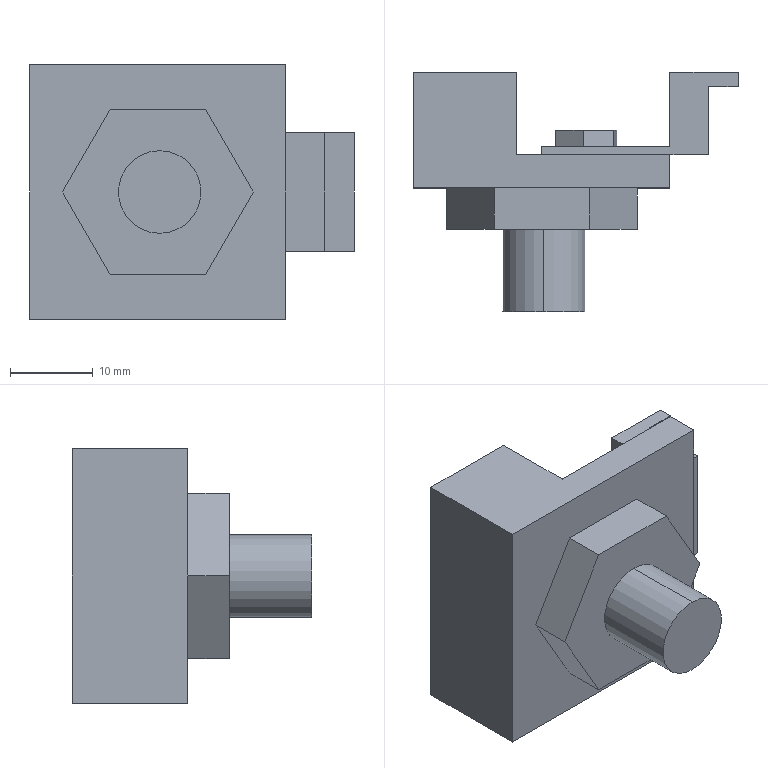Part | SolidWorks | features ICE 9, Extrusion 1 | 1 solid | 54 faces | box 39.277 x 29 x 30.752 mm | volume 9979 mm3 | plane 46 | cylinder 8 | commonest cylinder face diameters 8.542 x4 3.886 x2 10 x2
STEP:
#1=CARTESIAN_POINT('',(19.89,18.9,-1.943));
#2=VERTEX_POINT('',#1);
#3=CARTESIAN_POINT('',(18.72,18.9,1.551));
#4=VERTEX_POINT('',#3);
#5=CARTESIAN_POINT('',(19.89,18.9,0.));
#6=DIRECTION('',(0.,1.,0.));
#7=DIRECTION('',(0.,0.,1.));
#8=AXIS2_PLACEMENT_3D('',#5,#6,#7);
#9=CIRCLE('',#8,1.943);
#10=EDGE_CURVE('',#2,#4,#9,.T.);
#11=ORIENTED_EDGE('',*,*,#10,.F.);
#12=CARTESIAN_POINT('',(19.89,19.,-1.943));
#13=VERTEX_POINT('',#12);
#14=CARTESIAN_POINT('',(19.89,18.9,-1.943));
#15=DIRECTION('',(0.,1.,0.));
#16=VECTOR('',#15,1000.);
#17=LINE('',#14,#16);
#18=EDGE_CURVE('',#2,#13,#17,.T.);
#19=ORIENTED_EDGE('',*,*,#18,.T.);
#20=CARTESIAN_POINT('',(19.89,19.,1.943));
#21=VERTEX_POINT('',#20);
#22=CARTESIAN_POINT('',(19.89,19.,0.));
#23=DIRECTION('',(0.,1.,0.));
#24=DIRECTION('',(0.,0.,1.));
#25=AXIS2_PLACEMENT_3D('',#22,#23,#24);
#26=CIRCLE('',#25,1.943);
#27=EDGE_CURVE('',#13,#21,#26,.T.);
#28=ORIENTED_EDGE('',*,*,#27,.T.);
#29=CARTESIAN_POINT('',(19.89,18.9,1.943));
#30=VERTEX_POINT('',#29);
#31=CARTESIAN_POINT('',(19.89,18.9,1.943));
#32=DIRECTION('',(0.,1.,0.));
#33=VECTOR('',#32,1000.);
#34=LINE('',#31,#33);
#35=EDGE_CURVE('',#30,#21,#34,.T.);
#36=ORIENTED_EDGE('',*,*,#35,.F.);
#37=CARTESIAN_POINT('',(19.07,18.9,1.762));
#38=VERTEX_POINT('',#37);
#39=CARTESIAN_POINT('',(19.89,18.9,0.));
#40=DIRECTION('',(0.,1.,0.));
#41=DIRECTION('',(0.,0.,1.));
#42=AXIS2_PLACEMENT_3D('',#39,#40,#41);
#43=CIRCLE('',#42,1.943);
#44=EDGE_CURVE('',#38,#30,#43,.T.);
#45=ORIENTED_EDGE('',*,*,#44,.F.);
#46=CARTESIAN_POINT('',(18.89,18.9,1.666));
#47=VERTEX_POINT('',#46);
#48=CARTESIAN_POINT('',(19.89,18.9,0.));
#49=DIRECTION('',(0.,1.,0.));
#50=DIRECTION('',(0.,0.,1.));
#51=AXIS2_PLACEMENT_3D('',#48,#49,#50);
#52=CIRCLE('',#51,1.943);
#53=EDGE_CURVE('',#47,#38,#52,.T.);
#54=ORIENTED_EDGE('',*,*,#53,.F.);
#55=CARTESIAN_POINT('',(19.89,18.9,0.));
#56=DIRECTION('',(0.,1.,0.));
#57=DIRECTION('',(0.,0.,1.));
#58=AXIS2_PLACEMENT_3D('',#55,#56,#57);
#59=CIRCLE('',#58,1.943);
#60=EDGE_CURVE('',#4,#47,#59,.T.);
#61=ORIENTED_EDGE('',*,*,#60,.F.);
#62=EDGE_LOOP('',(#11,#19,#28,#36,#45,#54,#61));
#63=FACE_OUTER_BOUND('',#62,.T.);
#64=CARTESIAN_POINT('',(19.89,18.9,0.));
#65=DIRECTION('',(0.,1.,0.));
#66=DIRECTION('',(0.,0.,1.));
#67=AXIS2_PLACEMENT_3D('',#64,#65,#66);
#68=CYLINDRICAL_SURFACE('',#67,1.943);
#69=ADVANCED_FACE('',(#63),#68,.F.);
#70=CARTESIAN_POINT('',(-9.584,8.,-10.188));
#71=VERTEX_POINT('',#70);
#72=CARTESIAN_POINT('',(-9.584,8.,-1.646));
#73=VERTEX_POINT('',#72);
#74=CARTESIAN_POINT('',(-9.584,8.,-5.917));
#75=DIRECTION('',(0.,1.,0.));
#76=DIRECTION('',(0.,0.,1.));
#77=AXIS2_PLACEMENT_3D('',#74,#75,#76);
#78=CIRCLE('',#77,4.271);
#79=EDGE_CURVE('',#71,#73,#78,.T.);
#80=ORIENTED_EDGE('',*,*,#79,.F.);
#81=CARTESIAN_POINT('',(-9.584,19.,-10.188));
#82=VERTEX_POINT('',#81);
#83=CARTESIAN_POINT('',(-9.584,8.,-10.188));
#84=DIRECTION('',(0.,1.,0.));
#85=VECTOR('',#84,1000.);
#86=LINE('',#83,#85);
#87=EDGE_CURVE('',#71,#82,#86,.T.);
#88=ORIENTED_EDGE('',*,*,#87,.T.);
#89=CARTESIAN_POINT('',(-9.584,19.,-1.646));
#90=VERTEX_POINT('',#89);
#91=CARTESIAN_POINT('',(-9.584,19.,-5.917));
#92=DIRECTION('',(0.,1.,0.));
#93=DIRECTION('',(0.,0.,1.));
#94=AXIS2_PLACEMENT_3D('',#91,#92,#93);
#95=CIRCLE('',#94,4.271);
#96=EDGE_CURVE('',#82,#90,#95,.T.);
#97=ORIENTED_EDGE('',*,*,#96,.T.);
#98=CARTESIAN_POINT('',(-9.584,8.,-1.646));
#99=DIRECTION('',(0.,1.,0.));
#100=VECTOR('',#99,1000.);
#101=LINE('',#98,#100);
#102=EDGE_CURVE('',#73,#90,#101,.T.);
#103=ORIENTED_EDGE('',*,*,#102,.F.);
#104=EDGE_LOOP('',(#80,#88,#97,#103));
#105=FACE_OUTER_BOUND('',#104,.T.);
#106=CARTESIAN_POINT('',(-9.584,8.,-5.917));
#107=DIRECTION('',(0.,1.,0.));
#108=DIRECTION('',(0.,0.,1.));
#109=AXIS2_PLACEMENT_3D('',#106,#107,#108);
#110=CYLINDRICAL_SURFACE('',#109,4.271);
#111=ADVANCED_FACE('',(#105),#110,.F.);
#112=CARTESIAN_POINT('',(-9.584,8.,2.375));
#113=VERTEX_POINT('',#112);
#114=CARTESIAN_POINT('',(-9.584,8.,10.916));
#115=VERTEX_POINT('',#114);
#116=CARTESIAN_POINT('',(-9.584,8.,6.646));
#117=DIRECTION('',(0.,1.,0.));
#118=DIRECTION('',(0.,0.,1.));
#119=AXIS2_PLACEMENT_3D('',#116,#117,#118);
#120=CIRCLE('',#119,4.271);
#121=EDGE_CURVE('',#113,#115,#120,.T.);
#122=ORIENTED_EDGE('',*,*,#121,.F.);
#123=CARTESIAN_POINT('',(-9.584,19.,2.375));
#124=VERTEX_POINT('',#123);
#125=CARTESIAN_POINT('',(-9.584,8.,2.375));
#126=DIRECTION('',(0.,1.,0.));
#127=VECTOR('',#126,1000.);
#128=LINE('',#125,#127);
#129=EDGE_CURVE('',#113,#124,#128,.T.);
#130=ORIENTED_EDGE('',*,*,#129,.T.);
#131=CARTESIAN_POINT('',(-9.584,19.,10.916));
#132=VERTEX_POINT('',#131);
#133=CARTESIAN_POINT('',(-9.584,19.,6.646));
#134=DIRECTION('',(0.,1.,0.));
#135=DIRECTION('',(0.,0.,1.));
#136=AXIS2_PLACEMENT_3D('',#133,#134,#135);
#137=CIRCLE('',#136,4.271);
#138=EDGE_CURVE('',#124,#132,#137,.T.);
#139=ORIENTED_EDGE('',*,*,#138,.T.);
#140=CARTESIAN_POINT('',(-9.584,8.,10.916));
#141=DIRECTION('',(0.,1.,0.));
#142=VECTOR('',#141,1000.);
#143=LINE('',#140,#142);
#144=EDGE_CURVE('',#115,#132,#143,.T.);
#145=ORIENTED_EDGE('',*,*,#144,.F.);
#146=EDGE_LOOP('',(#122,#130,#139,#145));
#147=FACE_OUTER_BOUND('',#146,.T.);
#148=CARTESIAN_POINT('',(-9.584,8.,6.646));
#149=DIRECTION('',(0.,1.,0.));
#150=DIRECTION('',(0.,0.,1.));
#151=AXIS2_PLACEMENT_3D('',#148,#149,#150);
#152=CYLINDRICAL_SURFACE('',#151,4.271);
#153=ADVANCED_FACE('',(#147),#152,.F.);
#154=CARTESIAN_POINT('',(0.2348,-10.,-5.));
#155=VERTEX_POINT('',#154);
#156=CARTESIAN_POINT('',(0.2348,-10.,5.));
#157=VERTEX_POINT('',#156);
#158=CARTESIAN_POINT('',(0.2348,-10.,0.));
#159=DIRECTION('',(0.,-1.,0.));
#160=DIRECTION('',(0.,0.,-1.));
#161=AXIS2_PLACEMENT_3D('',#158,#159,#160);
#162=CIRCLE('',#161,5.);
#163=EDGE_CURVE('',#155,#157,#162,.T.);
#164=ORIENTED_EDGE('',*,*,#163,.F.);
#165=CARTESIAN_POINT('',(0.2348,0.,-5.));
#166=VERTEX_POINT('',#165);
#167=CARTESIAN_POINT('',(0.2348,-10.,-5.));
#168=DIRECTION('',(0.,1.,0.));
#169=VECTOR('',#168,1000.);
#170=LINE('',#167,#169);
#171=EDGE_CURVE('',#155,#166,#170,.T.);
#172=ORIENTED_EDGE('',*,*,#171,.T.);
#173=CARTESIAN_POINT('',(0.2348,0.,5.));
#174=VERTEX_POINT('',#173);
#175=CARTESIAN_POINT('',(0.2348,0.,0.));
#176=DIRECTION('',(0.,-1.,0.));
#177=DIRECTION('',(0.,0.,-1.));
#178=AXIS2_PLACEMENT_3D('',#175,#176,#177);
#179=CIRCLE('',#178,5.);
#180=EDGE_CURVE('',#166,#174,#179,.T.);
#181=ORIENTED_EDGE('',*,*,#180,.T.);
#182=CARTESIAN_POINT('',(0.2348,-10.,5.));
#183=DIRECTION('',(0.,1.,0.));
#184=VECTOR('',#183,1000.);
#185=LINE('',#182,#184);
#186=EDGE_CURVE('',#157,#174,#185,.T.);
#187=ORIENTED_EDGE('',*,*,#186,.F.);
#188=EDGE_LOOP('',(#164,#172,#181,#187));
#189=FACE_OUTER_BOUND('',#188,.T.);
#190=CARTESIAN_POINT('',(0.2348,-10.,0.));
#191=DIRECTION('',(0.,1.,0.));
#192=DIRECTION('',(0.,0.,1.));
#193=AXIS2_PLACEMENT_3D('',#190,#191,#192);
#194=CYLINDRICAL_SURFACE('',#193,5.);
#195=ADVANCED_FACE('',(#189),#194,.T.);
#196=CARTESIAN_POINT('',(15.495,10.,-7.2));
#197=VERTEX_POINT('',#196);
#198=CARTESIAN_POINT('',(15.495,10.,7.2));
#199=VERTEX_POINT('',#198);
#200=CARTESIAN_POINT('',(15.495,10.,-19.428));
#201=DIRECTION('',(0.,0.,1.));
#202=VECTOR('',#201,1000.);
#203=LINE('',#200,#202);
#204=EDGE_CURVE('',#197,#199,#203,.T.);
#205=ORIENTED_EDGE('',*,*,#204,.F.);
#206=CARTESIAN_POINT('',(0.,10.,-7.2));
#207=VERTEX_POINT('',#206);
#208=CARTESIAN_POINT('',(0.,10.,-7.2));
#209=DIRECTION('',(-1.,0.,0.));
#210=VECTOR('',#209,1000.);
#211=LINE('',#208,#210);
#212=EDGE_CURVE('',#197,#207,#211,.T.);
#213=ORIENTED_EDGE('',*,*,#212,.T.);
#214=CARTESIAN_POINT('',(0.,10.,7.2));
#215=VERTEX_POINT('',#214);
#216=CARTESIAN_POINT('',(0.,10.,-7.2));
#217=DIRECTION('',(0.,0.,1.));
#218=VECTOR('',#217,1000.);
#219=LINE('',#216,#218);
#220=EDGE_CURVE('',#207,#215,#219,.T.);
#221=ORIENTED_EDGE('',*,*,#220,.T.);
#222=CARTESIAN_POINT('',(0.,10.,7.2));
#223=DIRECTION('',(1.,0.,0.));
#224=VECTOR('',#223,1000.);
#225=LINE('',#222,#224);
#226=EDGE_CURVE('',#215,#199,#225,.T.);
#227=ORIENTED_EDGE('',*,*,#226,.T.);
#228=EDGE_LOOP('',(#205,#213,#221,#227));
#229=FACE_OUTER_BOUND('',#228,.T.);
#230=CARTESIAN_POINT('',(5.703,10.,-4.089));
#231=VERTEX_POINT('',#230);
#232=CARTESIAN_POINT('',(1.991,10.,-2.341));
#233=VERTEX_POINT('',#232);
#234=CARTESIAN_POINT('',(5.703,10.,-4.089));
#235=DIRECTION('',(-0.9047,0.,0.426));
#236=VECTOR('',#235,1000.);
#237=LINE('',#234,#236);
#238=EDGE_CURVE('',#231,#233,#237,.T.);
#239=ORIENTED_EDGE('',*,*,#238,.F.);
#240=CARTESIAN_POINT('',(9.073,10.,-1.748));
#241=VERTEX_POINT('',#240);
#242=CARTESIAN_POINT('',(9.073,10.,-1.748));
#243=DIRECTION('',(-0.8213,0.,-0.5705));
#244=VECTOR('',#243,1000.);
#245=LINE('',#242,#244);
#246=EDGE_CURVE('',#241,#231,#245,.T.);
#247=ORIENTED_EDGE('',*,*,#246,.F.);
#248=CARTESIAN_POINT('',(8.731,10.,2.341));
#249=VERTEX_POINT('',#248);
#250=CARTESIAN_POINT('',(8.731,10.,2.341));
#251=DIRECTION('',(0.0834,0.,-0.9965));
#252=VECTOR('',#251,1000.);
#253=LINE('',#250,#252);
#254=EDGE_CURVE('',#249,#241,#253,.T.);
#255=ORIENTED_EDGE('',*,*,#254,.F.);
#256=CARTESIAN_POINT('',(5.019,10.,4.089));
#257=VERTEX_POINT('',#256);
#258=CARTESIAN_POINT('',(5.019,10.,4.089));
#259=DIRECTION('',(0.9047,0.,-0.426));
#260=VECTOR('',#259,1000.);
#261=LINE('',#258,#260);
#262=EDGE_CURVE('',#257,#249,#261,.T.);
#263=ORIENTED_EDGE('',*,*,#262,.F.);
#264=CARTESIAN_POINT('',(1.649,10.,1.748));
#265=VERTEX_POINT('',#264);
#266=CARTESIAN_POINT('',(1.649,10.,1.748));
#267=DIRECTION('',(0.8213,0.,0.5705));
#268=VECTOR('',#267,1000.);
#269=LINE('',#266,#268);
#270=EDGE_CURVE('',#265,#257,#269,.T.);
#271=ORIENTED_EDGE('',*,*,#270,.F.);
#272=CARTESIAN_POINT('',(1.991,10.,-2.341));
#273=DIRECTION('',(-0.0834,0.,0.9965));
#274=VECTOR('',#273,1000.);
#275=LINE('',#272,#274);
#276=EDGE_CURVE('',#233,#265,#275,.T.);
#277=ORIENTED_EDGE('',*,*,#276,.F.);
#278=EDGE_LOOP('',(#239,#247,#255,#263,#271,#277));
#279=FACE_BOUND('',#278,.T.);
#280=CARTESIAN_POINT('',(0.,10.,0.));
#281=DIRECTION('',(0.,1.,0.));
#282=DIRECTION('',(0.,0.,1.));
#283=AXIS2_PLACEMENT_3D('',#280,#281,#282);
#284=PLANE('',#283);
#285=ADVANCED_FACE('',(#229,#279),#284,.T.);
#286=CARTESIAN_POINT('',(20.709,18.9,-1.762));
#287=VERTEX_POINT('',#286);
#288=CARTESIAN_POINT('',(19.714,18.9,-0.1053));
#289=DIRECTION('',(-0.5147,0.,0.8574));
#290=VECTOR('',#289,1000.);
#291=LINE('',#288,#290);
#292=EDGE_CURVE('',#287,#4,#291,.T.);
#293=ORIENTED_EDGE('',*,*,#292,.F.);
#294=CARTESIAN_POINT('',(19.89,18.9,0.));
#295=DIRECTION('',(0.,1.,0.));
#296=DIRECTION('',(0.,0.,1.));
#297=AXIS2_PLACEMENT_3D('',#294,#295,#296);
#298=CIRCLE('',#297,1.943);
#299=EDGE_CURVE('',#287,#2,#298,.T.);
#300=ORIENTED_EDGE('',*,*,#299,.T.);
#301=ORIENTED_EDGE('',*,*,#10,.T.);
#302=EDGE_LOOP('',(#293,#300,#301));
#303=FACE_OUTER_BOUND('',#302,.T.);
#304=CARTESIAN_POINT('',(19.89,18.9,0.));
#305=DIRECTION('',(0.,1.,0.));
#306=DIRECTION('',(0.,0.,1.));
#307=AXIS2_PLACEMENT_3D('',#304,#305,#306);
#308=PLANE('',#307);
#309=ADVANCED_FACE('',(#303),#308,.T.);
#310=CARTESIAN_POINT('',(15.504,9.,-7.2));
#311=VERTEX_POINT('',#310);
#312=CARTESIAN_POINT('',(0.,9.,-7.2));
#313=VERTEX_POINT('',#312);
#314=CARTESIAN_POINT('',(0.,9.,-7.2));
#315=DIRECTION('',(-1.,0.,0.));
#316=VECTOR('',#315,1000.);
#317=LINE('',#314,#316);
#318=EDGE_CURVE('',#311,#313,#317,.T.);
#319=ORIENTED_EDGE('',*,*,#318,.F.);
#320=CARTESIAN_POINT('',(15.504,9.,-15.376));
#321=VERTEX_POINT('',#320);
#322=CARTESIAN_POINT('',(15.504,9.,15.376));
#323=DIRECTION('',(0.,0.,-1.));
#324=VECTOR('',#323,1000.);
#325=LINE('',#322,#324);
#326=EDGE_CURVE('',#311,#321,#325,.T.);
#327=ORIENTED_EDGE('',*,*,#326,.T.);
#328=CARTESIAN_POINT('',(-3.031,9.,-15.376));
#329=VERTEX_POINT('',#328);
#330=CARTESIAN_POINT('',(-15.504,9.,-15.376));
#331=DIRECTION('',(-1.,0.,0.));
#332=VECTOR('',#331,1000.);
#333=LINE('',#330,#332);
#334=EDGE_CURVE('',#321,#329,#333,.T.);
#335=ORIENTED_EDGE('',*,*,#334,.T.);
#336=CARTESIAN_POINT('',(-3.031,9.,15.376));
#337=VERTEX_POINT('',#336);
#338=CARTESIAN_POINT('',(-3.031,9.,-15.376));
#339=DIRECTION('',(0.,0.,-1.));
#340=VECTOR('',#339,1000.);
#341=LINE('',#338,#340);
#342=EDGE_CURVE('',#337,#329,#341,.T.);
#343=ORIENTED_EDGE('',*,*,#342,.F.);
#344=CARTESIAN_POINT('',(15.504,9.,15.376));
#345=VERTEX_POINT('',#344);
#346=CARTESIAN_POINT('',(-15.504,9.,15.376));
#347=DIRECTION('',(1.,0.,0.));
#348=VECTOR('',#347,1000.);
#349=LINE('',#346,#348);
#350=EDGE_CURVE('',#337,#345,#349,.T.);
#351=ORIENTED_EDGE('',*,*,#350,.T.);
#352=CARTESIAN_POINT('',(15.504,9.,7.2));
#353=VERTEX_POINT('',#352);
#354=CARTESIAN_POINT('',(15.504,9.,15.376));
#355=DIRECTION('',(0.,0.,-1.));
#356=VECTOR('',#355,1000.);
#357=LINE('',#354,#356);
#358=EDGE_CURVE('',#345,#353,#357,.T.);
#359=ORIENTED_EDGE('',*,*,#358,.T.);
#360=CARTESIAN_POINT('',(0.,9.,7.2));
#361=VERTEX_POINT('',#360);
#362=CARTESIAN_POINT('',(0.,9.,7.2));
#363=DIRECTION('',(1.,0.,0.));
#364=VECTOR('',#363,1000.);
#365=LINE('',#362,#364);
#366=EDGE_CURVE('',#361,#353,#365,.T.);
#367=ORIENTED_EDGE('',*,*,#366,.F.);
#368=CARTESIAN_POINT('',(0.,9.,-7.2));
#369=DIRECTION('',(0.,0.,1.));
#370=VECTOR('',#369,1000.);
#371=LINE('',#368,#370);
#372=EDGE_CURVE('',#313,#361,#371,.T.);
#373=ORIENTED_EDGE('',*,*,#372,.F.);
#374=EDGE_LOOP('',(#319,#327,#335,#343,#351,#359,#367,#373));
#375=FACE_OUTER_BOUND('',#374,.T.);
#376=CARTESIAN_POINT('',(0.,9.,0.));
#377=DIRECTION('',(0.,-1.,0.));
#378=DIRECTION('',(0.,0.,-1.));
#379=AXIS2_PLACEMENT_3D('',#376,#377,#378);
#380=PLANE('',#379);
#381=ADVANCED_FACE('',(#375),#380,.F.);
#382=CARTESIAN_POINT('',(11.547,0.,0.));
#383=VERTEX_POINT('',#382);
#384=CARTESIAN_POINT('',(5.774,0.,-10.));
#385=VERTEX_POINT('',#384);
#386=CARTESIAN_POINT('',(11.547,0.,0.));
#387=DIRECTION('',(-0.5,0.,-0.866));
#388=VECTOR('',#387,1000.);
#389=LINE('',#386,#388);
#390=EDGE_CURVE('',#383,#385,#389,.T.);
#391=ORIENTED_EDGE('',*,*,#390,.T.);
#392=CARTESIAN_POINT('',(5.774,5.,-10.));
#393=VERTEX_POINT('',#392);
#394=CARTESIAN_POINT('',(5.774,5.,-10.));
#395=DIRECTION('',(0.,-1.,0.));
#396=VECTOR('',#395,1000.);
#397=LINE('',#394,#396);
#398=EDGE_CURVE('',#393,#385,#397,.T.);
#399=ORIENTED_EDGE('',*,*,#398,.F.);
#400=CARTESIAN_POINT('',(11.547,5.,0.));
#401=VERTEX_POINT('',#400);
#402=CARTESIAN_POINT('',(11.547,5.,0.));
#403=DIRECTION('',(-0.5,0.,-0.866));
#404=VECTOR('',#403,1000.);
#405=LINE('',#402,#404);
#406=EDGE_CURVE('',#401,#393,#405,.T.);
#407=ORIENTED_EDGE('',*,*,#406,.F.);
#408=CARTESIAN_POINT('',(11.547,5.,0.));
#409=DIRECTION('',(0.,-1.,0.));
#410=VECTOR('',#409,1000.);
#411=LINE('',#408,#410);
#412=EDGE_CURVE('',#401,#383,#411,.T.);
#413=ORIENTED_EDGE('',*,*,#412,.T.);
#414=EDGE_LOOP('',(#391,#399,#407,#413));
#415=FACE_OUTER_BOUND('',#414,.T.);
#416=CARTESIAN_POINT('',(11.547,5.,0.));
#417=DIRECTION('',(-0.866,0.,0.5));
#418=DIRECTION('',(0.5,0.,0.866));
#419=AXIS2_PLACEMENT_3D('',#416,#417,#418);
#420=PLANE('',#419);
#421=ADVANCED_FACE('',(#415),#420,.F.);
#422=CARTESIAN_POINT('',(-5.774,0.,-10.));
#423=VERTEX_POINT('',#422);
#424=CARTESIAN_POINT('',(5.774,0.,-10.));
#425=DIRECTION('',(-1.,0.,0.));
#426=VECTOR('',#425,1000.);
#427=LINE('',#424,#426);
#428=EDGE_CURVE('',#385,#423,#427,.T.);
#429=ORIENTED_EDGE('',*,*,#428,.T.);
#430=CARTESIAN_POINT('',(-5.774,5.,-10.));
#431=VERTEX_POINT('',#430);
#432=CARTESIAN_POINT('',(-5.774,5.,-10.));
#433=DIRECTION('',(0.,-1.,0.));
#434=VECTOR('',#433,1000.);
#435=LINE('',#432,#434);
#436=EDGE_CURVE('',#431,#423,#435,.T.);
#437=ORIENTED_EDGE('',*,*,#436,.F.);
#438=CARTESIAN_POINT('',(5.774,5.,-10.));
#439=DIRECTION('',(-1.,0.,0.));
#440=VECTOR('',#439,1000.);
#441=LINE('',#438,#440);
#442=EDGE_CURVE('',#393,#431,#441,.T.);
#443=ORIENTED_EDGE('',*,*,#442,.F.);
#444=ORIENTED_EDGE('',*,*,#398,.T.);
#445=EDGE_LOOP('',(#429,#437,#443,#444));
#446=FACE_OUTER_BOUND('',#445,.T.);
#447=CARTESIAN_POINT('',(5.774,5.,-10.));
#448=DIRECTION('',(0.,0.,1.));
#449=DIRECTION('',(1.,0.,0.));
#450=AXIS2_PLACEMENT_3D('',#447,#448,#449);
#451=PLANE('',#450);
#452=ADVANCED_FACE('',(#446),#451,.F.);
#453=CARTESIAN_POINT('',(-11.547,0.,0.));
#454=VERTEX_POINT('',#453);
#455=CARTESIAN_POINT('',(-5.774,0.,-10.));
#456=DIRECTION('',(-0.5,0.,0.866));
#457=VECTOR('',#456,1000.);
#458=LINE('',#455,#457);
#459=EDGE_CURVE('',#423,#454,#458,.T.);
#460=ORIENTED_EDGE('',*,*,#459,.T.);
#461=CARTESIAN_POINT('',(-11.547,5.,0.));
#462=VERTEX_POINT('',#461);
#463=CARTESIAN_POINT('',(-11.547,5.,0.));
#464=DIRECTION('',(0.,-1.,0.));
#465=VECTOR('',#464,1000.);
#466=LINE('',#463,#465);
#467=EDGE_CURVE('',#462,#454,#466,.T.);
#468=ORIENTED_EDGE('',*,*,#467,.F.);
#469=CARTESIAN_POINT('',(-5.774,5.,-10.));
#470=DIRECTION('',(-0.5,0.,0.866));
#471=VECTOR('',#470,1000.);
#472=LINE('',#469,#471);
#473=EDGE_CURVE('',#431,#462,#472,.T.);
#474=ORIENTED_EDGE('',*,*,#473,.F.);
#475=ORIENTED_EDGE('',*,*,#436,.T.);
#476=EDGE_LOOP('',(#460,#468,#474,#475));
#477=FACE_OUTER_BOUND('',#476,.T.);
#478=CARTESIAN_POINT('',(-5.774,5.,-10.));
#479=DIRECTION('',(0.866,0.,0.5));
#480=DIRECTION('',(0.5,0.,-0.866));
#481=AXIS2_PLACEMENT_3D('',#478,#479,#480);
#482=PLANE('',#481);
#483=ADVANCED_FACE('',(#477),#482,.F.);
#484=CARTESIAN_POINT('',(-5.774,0.,10.));
#485=VERTEX_POINT('',#484);
#486=CARTESIAN_POINT('',(-11.547,0.,0.));
#487=DIRECTION('',(0.5,0.,0.866));
#488=VECTOR('',#487,1000.);
#489=LINE('',#486,#488);
#490=EDGE_CURVE('',#454,#485,#489,.T.);
#491=ORIENTED_EDGE('',*,*,#490,.T.);
#492=CARTESIAN_POINT('',(-5.774,5.,10.));
#493=VERTEX_POINT('',#492);
#494=CARTESIAN_POINT('',(-5.774,5.,10.));
#495=DIRECTION('',(0.,-1.,0.));
#496=VECTOR('',#495,1000.);
#497=LINE('',#494,#496);
#498=EDGE_CURVE('',#493,#485,#497,.T.);
#499=ORIENTED_EDGE('',*,*,#498,.F.);
#500=CARTESIAN_POINT('',(-11.547,5.,0.));
#501=DIRECTION('',(0.5,0.,0.866));
#502=VECTOR('',#501,1000.);
#503=LINE('',#500,#502);
#504=EDGE_CURVE('',#462,#493,#503,.T.);
#505=ORIENTED_EDGE('',*,*,#504,.F.);
#506=ORIENTED_EDGE('',*,*,#467,.T.);
#507=EDGE_LOOP('',(#491,#499,#505,#506));
#508=FACE_OUTER_BOUND('',#507,.T.);
#509=CARTESIAN_POINT('',(-11.547,5.,0.));
#510=DIRECTION('',(0.866,0.,-0.5));
#511=DIRECTION('',(-0.5,0.,-0.866));
#512=AXIS2_PLACEMENT_3D('',#509,#510,#511);
#513=PLANE('',#512);
#514=ADVANCED_FACE('',(#508),#513,.F.);
#515=CARTESIAN_POINT('',(5.774,0.,10.));
#516=VERTEX_POINT('',#515);
#517=CARTESIAN_POINT('',(-5.774,0.,10.));
#518=DIRECTION('',(1.,0.,0.));
#519=VECTOR('',#518,1000.);
#520=LINE('',#517,#519);
#521=EDGE_CURVE('',#485,#516,#520,.T.);
#522=ORIENTED_EDGE('',*,*,#521,.T.);
#523=CARTESIAN_POINT('',(5.774,5.,10.));
#524=VERTEX_POINT('',#523);
#525=CARTESIAN_POINT('',(5.774,5.,10.));
#526=DIRECTION('',(0.,-1.,0.));
#527=VECTOR('',#526,1000.);
#528=LINE('',#525,#527);
#529=EDGE_CURVE('',#524,#516,#528,.T.);
#530=ORIENTED_EDGE('',*,*,#529,.F.);
#531=CARTESIAN_POINT('',(-5.774,5.,10.));
#532=DIRECTION('',(1.,0.,0.));
#533=VECTOR('',#532,1000.);
#534=LINE('',#531,#533);
#535=EDGE_CURVE('',#493,#524,#534,.T.);
#536=ORIENTED_EDGE('',*,*,#535,.F.);
#537=ORIENTED_EDGE('',*,*,#498,.T.);
#538=EDGE_LOOP('',(#522,#530,#536,#537));
#539=FACE_OUTER_BOUND('',#538,.T.);
#540=CARTESIAN_POINT('',(-5.774,5.,10.));
#541=DIRECTION('',(0.,0.,-1.));
#542=DIRECTION('',(-1.,0.,0.));
#543=AXIS2_PLACEMENT_3D('',#540,#541,#542);
#544=PLANE('',#543);
#545=ADVANCED_FACE('',(#539),#544,.F.);
#546=CARTESIAN_POINT('',(5.774,0.,10.));
#547=DIRECTION('',(0.5,0.,-0.866));
#548=VECTOR('',#547,1000.);
#549=LINE('',#546,#548);
#550=EDGE_CURVE('',#516,#383,#549,.T.);
#551=ORIENTED_EDGE('',*,*,#550,.T.);
#552=ORIENTED_EDGE('',*,*,#412,.F.);
#553=CARTESIAN_POINT('',(5.774,5.,10.));
#554=DIRECTION('',(0.5,0.,-0.866));
#555=VECTOR('',#554,1000.);
#556=LINE('',#553,#555);
#557=EDGE_CURVE('',#524,#401,#556,.T.);
#558=ORIENTED_EDGE('',*,*,#557,.F.);
#559=ORIENTED_EDGE('',*,*,#529,.T.);
#560=EDGE_LOOP('',(#551,#552,#558,#559));
#561=FACE_OUTER_BOUND('',#560,.T.);
#562=CARTESIAN_POINT('',(5.774,5.,10.));
#563=DIRECTION('',(-0.866,0.,-0.5));
#564=DIRECTION('',(-0.5,0.,0.866));
#565=AXIS2_PLACEMENT_3D('',#562,#563,#564);
#566=PLANE('',#565);
#567=ADVANCED_FACE('',(#561),#566,.F.);
#568=CARTESIAN_POINT('',(0.2348,0.,0.));
#569=DIRECTION('',(0.,-1.,0.));
#570=DIRECTION('',(0.,0.,-1.));
#571=AXIS2_PLACEMENT_3D('',#568,#569,#570);
#572=CIRCLE('',#571,5.);
#573=EDGE_CURVE('',#174,#166,#572,.T.);
#574=ORIENTED_EDGE('',*,*,#573,.F.);
#575=ORIENTED_EDGE('',*,*,#180,.F.);
#576=EDGE_LOOP('',(#574,#575));
#577=FACE_BOUND('',#576,.T.);
#578=ORIENTED_EDGE('',*,*,#390,.F.);
#579=ORIENTED_EDGE('',*,*,#550,.F.);
#580=ORIENTED_EDGE('',*,*,#521,.F.);
#581=ORIENTED_EDGE('',*,*,#490,.F.);
#582=ORIENTED_EDGE('',*,*,#459,.F.);
#583=ORIENTED_EDGE('',*,*,#428,.F.);
#584=EDGE_LOOP('',(#578,#579,#580,#581,#582,#583));
#585=FACE_OUTER_BOUND('',#584,.T.);
#586=CARTESIAN_POINT('',(0.,0.,0.));
#587=DIRECTION('',(0.,1.,0.));
#588=DIRECTION('',(0.,0.,1.));
#589=AXIS2_PLACEMENT_3D('',#586,#587,#588);
#590=PLANE('',#589);
#591=ADVANCED_FACE('',(#577,#585),#590,.F.);
#592=ORIENTED_EDGE('',*,*,#171,.F.);
#593=CARTESIAN_POINT('',(0.2348,-10.,0.));
#594=DIRECTION('',(0.,-1.,0.));
#595=DIRECTION('',(0.,0.,-1.));
#596=AXIS2_PLACEMENT_3D('',#593,#594,#595);
#597=CIRCLE('',#596,5.);
#598=EDGE_CURVE('',#157,#155,#597,.T.);
#599=ORIENTED_EDGE('',*,*,#598,.F.);
#600=ORIENTED_EDGE('',*,*,#186,.T.);
#601=ORIENTED_EDGE('',*,*,#573,.T.);
#602=EDGE_LOOP('',(#592,#599,#600,#601));
#603=FACE_OUTER_BOUND('',#602,.T.);
#604=CARTESIAN_POINT('',(0.2348,-10.,0.));
#605=DIRECTION('',(0.,1.,0.));
#606=DIRECTION('',(0.,0.,1.));
#607=AXIS2_PLACEMENT_3D('',#604,#605,#606);
#608=CYLINDRICAL_SURFACE('',#607,5.);
#609=ADVANCED_FACE('',(#603),#608,.T.);
#610=ORIENTED_EDGE('',*,*,#598,.T.);
#611=ORIENTED_EDGE('',*,*,#163,.T.);
#612=EDGE_LOOP('',(#610,#611));
#613=FACE_OUTER_BOUND('',#612,.T.);
#614=CARTESIAN_POINT('',(0.2348,-10.,0.));
#615=DIRECTION('',(0.,-1.,0.));
#616=DIRECTION('',(0.,0.,-1.));
#617=AXIS2_PLACEMENT_3D('',#614,#615,#616);
#618=PLANE('',#617);
#619=ADVANCED_FACE('',(#613),#618,.T.);
#620=CARTESIAN_POINT('',(15.504,5.,15.376));
#621=VERTEX_POINT('',#620);
#622=CARTESIAN_POINT('',(15.504,5.,-15.376));
#623=VERTEX_POINT('',#622);
#624=CARTESIAN_POINT('',(15.504,5.,15.376));
#625=DIRECTION('',(0.,0.,-1.));
#626=VECTOR('',#625,1000.);
#627=LINE('',#624,#626);
#628=EDGE_CURVE('',#621,#623,#627,.T.);
#629=ORIENTED_EDGE('',*,*,#628,.T.);
#630=CARTESIAN_POINT('',(15.504,9.,-15.376));
#631=DIRECTION('',(0.,-1.,0.));
#632=VECTOR('',#631,1000.);
#633=LINE('',#630,#632);
#634=EDGE_CURVE('',#321,#623,#633,.T.);
#635=ORIENTED_EDGE('',*,*,#634,.F.);
#636=ORIENTED_EDGE('',*,*,#326,.F.);
#637=CARTESIAN_POINT('',(15.504,9.,15.376));
#638=DIRECTION('',(0.,0.,-1.));
#639=VECTOR('',#638,1000.);
#640=LINE('',#637,#639);
#641=EDGE_CURVE('',#353,#311,#640,.T.);
#642=ORIENTED_EDGE('',*,*,#641,.F.);
#643=ORIENTED_EDGE('',*,*,#358,.F.);
#644=CARTESIAN_POINT('',(15.504,9.,15.376));
#645=DIRECTION('',(0.,-1.,0.));
#646=VECTOR('',#645,1000.);
#647=LINE('',#644,#646);
#648=EDGE_CURVE('',#345,#621,#647,.T.);
#649=ORIENTED_EDGE('',*,*,#648,.T.);
#650=EDGE_LOOP('',(#629,#635,#636,#642,#643,#649));
#651=FACE_OUTER_BOUND('',#650,.T.);
#652=CARTESIAN_POINT('',(15.504,9.,15.376));
#653=DIRECTION('',(-1.,0.,0.));
#654=DIRECTION('',(0.,0.,1.));
#655=AXIS2_PLACEMENT_3D('',#652,#653,#654);
#656=PLANE('',#655);
#657=ADVANCED_FACE('',(#651),#656,.F.);
#658=CARTESIAN_POINT('',(-15.504,5.,-15.376));
#659=VERTEX_POINT('',#658);
#660=CARTESIAN_POINT('',(-15.504,5.,-15.376));
#661=DIRECTION('',(-1.,0.,0.));
#662=VECTOR('',#661,1000.);
#663=LINE('',#660,#662);
#664=EDGE_CURVE('',#623,#659,#663,.T.);
#665=ORIENTED_EDGE('',*,*,#664,.T.);
#666=CARTESIAN_POINT('',(-15.504,19.,-15.376));
#667=VERTEX_POINT('',#666);
#668=CARTESIAN_POINT('',(-15.504,9.,-15.376));
#669=DIRECTION('',(0.,-1.,0.));
#670=VECTOR('',#669,1000.);
#671=LINE('',#668,#670);
#672=EDGE_CURVE('',#667,#659,#671,.T.);
#673=ORIENTED_EDGE('',*,*,#672,.F.);
#674=CARTESIAN_POINT('',(-3.031,19.,-15.376));
#675=VERTEX_POINT('',#674);
#676=CARTESIAN_POINT('',(-15.504,19.,-15.376));
#677=DIRECTION('',(-1.,0.,0.));
#678=VECTOR('',#677,1000.);
#679=LINE('',#676,#678);
#680=EDGE_CURVE('',#675,#667,#679,.T.);
#681=ORIENTED_EDGE('',*,*,#680,.F.);
#682=CARTESIAN_POINT('',(-3.031,19.,-15.376));
#683=DIRECTION('',(0.,-1.,0.));
#684=VECTOR('',#683,1000.);
#685=LINE('',#682,#684);
#686=EDGE_CURVE('',#675,#329,#685,.T.);
#687=ORIENTED_EDGE('',*,*,#686,.T.);
#688=ORIENTED_EDGE('',*,*,#334,.F.);
#689=ORIENTED_EDGE('',*,*,#634,.T.);
#690=EDGE_LOOP('',(#665,#673,#681,#687,#688,#689));
#691=FACE_OUTER_BOUND('',#690,.T.);
#692=CARTESIAN_POINT('',(-15.504,9.,-15.376));
#693=DIRECTION('',(0.,0.,1.));
#694=DIRECTION('',(1.,0.,0.));
#695=AXIS2_PLACEMENT_3D('',#692,#693,#694);
#696=PLANE('',#695);
#697=ADVANCED_FACE('',(#691),#696,.F.);
#698=CARTESIAN_POINT('',(-15.504,5.,15.376));
#699=VERTEX_POINT('',#698);
#700=CARTESIAN_POINT('',(-15.504,5.,15.376));
#701=DIRECTION('',(0.,0.,1.));
#702=VECTOR('',#701,1000.);
#703=LINE('',#700,#702);
#704=EDGE_CURVE('',#659,#699,#703,.T.);
#705=ORIENTED_EDGE('',*,*,#704,.T.);
#706=CARTESIAN_POINT('',(-15.504,19.,15.376));
#707=VERTEX_POINT('',#706);
#708=CARTESIAN_POINT('',(-15.504,9.,15.376));
#709=DIRECTION('',(0.,-1.,0.));
#710=VECTOR('',#709,1000.);
#711=LINE('',#708,#710);
#712=EDGE_CURVE('',#707,#699,#711,.T.);
#713=ORIENTED_EDGE('',*,*,#712,.F.);
#714=CARTESIAN_POINT('',(-15.504,19.,-15.376));
#715=DIRECTION('',(0.,0.,1.));
#716=VECTOR('',#715,1000.);
#717=LINE('',#714,#716);
#718=EDGE_CURVE('',#667,#707,#717,.T.);
#719=ORIENTED_EDGE('',*,*,#718,.F.);
#720=ORIENTED_EDGE('',*,*,#672,.T.);
#721=EDGE_LOOP('',(#705,#713,#719,#720));
#722=FACE_OUTER_BOUND('',#721,.T.);
#723=CARTESIAN_POINT('',(-15.504,9.,15.376));
#724=DIRECTION('',(1.,0.,0.));
#725=DIRECTION('',(0.,0.,-1.));
#726=AXIS2_PLACEMENT_3D('',#723,#724,#725);
#727=PLANE('',#726);
#728=ADVANCED_FACE('',(#722),#727,.F.);
#729=CARTESIAN_POINT('',(-15.504,5.,15.376));
#730=DIRECTION('',(1.,0.,0.));
#731=VECTOR('',#730,1000.);
#732=LINE('',#729,#731);
#733=EDGE_CURVE('',#699,#621,#732,.T.);
#734=ORIENTED_EDGE('',*,*,#733,.T.);
#735=ORIENTED_EDGE('',*,*,#648,.F.);
#736=ORIENTED_EDGE('',*,*,#350,.F.);
#737=CARTESIAN_POINT('',(-3.031,19.,15.376));
#738=VERTEX_POINT('',#737);
#739=CARTESIAN_POINT('',(-3.031,19.,15.376));
#740=DIRECTION('',(0.,-1.,0.));
#741=VECTOR('',#740,1000.);
#742=LINE('',#739,#741);
#743=EDGE_CURVE('',#738,#337,#742,.T.);
#744=ORIENTED_EDGE('',*,*,#743,.F.);
#745=CARTESIAN_POINT('',(-15.504,19.,15.376));
#746=DIRECTION('',(1.,0.,0.));
#747=VECTOR('',#746,1000.);
#748=LINE('',#745,#747);
#749=EDGE_CURVE('',#707,#738,#748,.T.);
#750=ORIENTED_EDGE('',*,*,#749,.F.);
#751=ORIENTED_EDGE('',*,*,#712,.T.);
#752=EDGE_LOOP('',(#734,#735,#736,#744,#750,#751));
#753=FACE_OUTER_BOUND('',#752,.T.);
#754=CARTESIAN_POINT('',(-15.504,9.,15.376));
#755=DIRECTION('',(0.,0.,-1.));
#756=DIRECTION('',(-1.,0.,0.));
#757=AXIS2_PLACEMENT_3D('',#754,#755,#756);
#758=PLANE('',#757);
#759=ADVANCED_FACE('',(#753),#758,.F.);
#760=ORIENTED_EDGE('',*,*,#557,.T.);
#761=ORIENTED_EDGE('',*,*,#406,.T.);
#762=ORIENTED_EDGE('',*,*,#442,.T.);
#763=ORIENTED_EDGE('',*,*,#473,.T.);
#764=ORIENTED_EDGE('',*,*,#504,.T.);
#765=ORIENTED_EDGE('',*,*,#535,.T.);
#766=EDGE_LOOP('',(#760,#761,#762,#763,#764,#765));
#767=FACE_BOUND('',#766,.T.);
#768=ORIENTED_EDGE('',*,*,#628,.F.);
#769=ORIENTED_EDGE('',*,*,#733,.F.);
#770=ORIENTED_EDGE('',*,*,#704,.F.);
#771=ORIENTED_EDGE('',*,*,#664,.F.);
#772=EDGE_LOOP('',(#768,#769,#770,#771));
#773=FACE_OUTER_BOUND('',#772,.T.);
#774=CARTESIAN_POINT('',(0.,5.,0.));
#775=DIRECTION('',(0.,-1.,0.));
#776=DIRECTION('',(0.,0.,-1.));
#777=AXIS2_PLACEMENT_3D('',#774,#775,#776);
#778=PLANE('',#777);
#779=ADVANCED_FACE('',(#767,#773),#778,.T.);
#780=ORIENTED_EDGE('',*,*,#342,.T.);
#781=ORIENTED_EDGE('',*,*,#686,.F.);
#782=CARTESIAN_POINT('',(-3.031,19.,-15.376));
#783=DIRECTION('',(0.,0.,-1.));
#784=VECTOR('',#783,1000.);
#785=LINE('',#782,#784);
#786=EDGE_CURVE('',#738,#675,#785,.T.);
#787=ORIENTED_EDGE('',*,*,#786,.F.);
#788=ORIENTED_EDGE('',*,*,#743,.T.);
#789=EDGE_LOOP('',(#780,#781,#787,#788));
#790=FACE_OUTER_BOUND('',#789,.T.);
#791=CARTESIAN_POINT('',(-3.031,19.,-15.376));
#792=DIRECTION('',(-1.,0.,0.));
#793=DIRECTION('',(0.,0.,1.));
#794=AXIS2_PLACEMENT_3D('',#791,#792,#793);
#795=PLANE('',#794);
#796=ADVANCED_FACE('',(#790),#795,.F.);
#797=CARTESIAN_POINT('',(-9.584,19.,-5.917));
#798=DIRECTION('',(0.,1.,0.));
#799=DIRECTION('',(0.,0.,1.));
#800=AXIS2_PLACEMENT_3D('',#797,#798,#799);
#801=CIRCLE('',#800,4.271);
#802=EDGE_CURVE('',#90,#82,#801,.T.);
#803=ORIENTED_EDGE('',*,*,#802,.F.);
#804=ORIENTED_EDGE('',*,*,#96,.F.);
#805=EDGE_LOOP('',(#803,#804));
#806=FACE_BOUND('',#805,.T.);
#807=CARTESIAN_POINT('',(-9.584,19.,6.646));
#808=DIRECTION('',(0.,1.,0.));
#809=DIRECTION('',(0.,0.,1.));
#810=AXIS2_PLACEMENT_3D('',#807,#808,#809);
#811=CIRCLE('',#810,4.271);
#812=EDGE_CURVE('',#132,#124,#811,.T.);
#813=ORIENTED_EDGE('',*,*,#812,.F.);
#814=ORIENTED_EDGE('',*,*,#138,.F.);
#815=EDGE_LOOP('',(#813,#814));
#816=FACE_BOUND('',#815,.T.);
#817=ORIENTED_EDGE('',*,*,#718,.T.);
#818=ORIENTED_EDGE('',*,*,#749,.T.);
#819=ORIENTED_EDGE('',*,*,#786,.T.);
#820=ORIENTED_EDGE('',*,*,#680,.T.);
#821=EDGE_LOOP('',(#817,#818,#819,#820));
#822=FACE_OUTER_BOUND('',#821,.T.);
#823=CARTESIAN_POINT('',(0.,19.,0.));
#824=DIRECTION('',(0.,1.,0.));
#825=DIRECTION('',(0.,0.,1.));
#826=AXIS2_PLACEMENT_3D('',#823,#824,#825);
#827=PLANE('',#826);
#828=ADVANCED_FACE('',(#806,#816,#822),#827,.T.);
#829=CARTESIAN_POINT('',(20.18,9.,7.2));
#830=VERTEX_POINT('',#829);
#831=CARTESIAN_POINT('',(0.,9.,7.2));
#832=DIRECTION('',(1.,0.,0.));
#833=VECTOR('',#832,1000.);
#834=LINE('',#831,#833);
#835=EDGE_CURVE('',#353,#830,#834,.T.);
#836=ORIENTED_EDGE('',*,*,#835,.F.);
#837=ORIENTED_EDGE('',*,*,#641,.T.);
#838=CARTESIAN_POINT('',(20.18,9.,-7.2));
#839=VERTEX_POINT('',#838);
#840=CARTESIAN_POINT('',(0.,9.,-7.2));
#841=DIRECTION('',(-1.,0.,0.));
#842=VECTOR('',#841,1000.);
#843=LINE('',#840,#842);
#844=EDGE_CURVE('',#839,#311,#843,.T.);
#845=ORIENTED_EDGE('',*,*,#844,.F.);
#846=CARTESIAN_POINT('',(20.18,9.,-7.2));
#847=DIRECTION('',(0.,0.,-1.));
#848=VECTOR('',#847,1000.);
#849=LINE('',#846,#848);
#850=EDGE_CURVE('',#830,#839,#849,.T.);
#851=ORIENTED_EDGE('',*,*,#850,.F.);
#852=EDGE_LOOP('',(#836,#837,#845,#851));
#853=FACE_OUTER_BOUND('',#852,.T.);
#854=CARTESIAN_POINT('',(0.,9.,0.));
#855=DIRECTION('',(0.,1.,0.));
#856=DIRECTION('',(0.,0.,1.));
#857=AXIS2_PLACEMENT_3D('',#854,#855,#856);
#858=PLANE('',#857);
#859=ADVANCED_FACE('',(#853),#858,.F.);
#860=ORIENTED_EDGE('',*,*,#850,.T.);
#861=CARTESIAN_POINT('',(20.18,17.284,-7.2));
#862=VERTEX_POINT('',#861);
#863=CARTESIAN_POINT('',(20.18,10.,-7.2));
#864=DIRECTION('',(0.,-1.,0.));
#865=VECTOR('',#864,1000.);
#866=LINE('',#863,#865);
#867=EDGE_CURVE('',#862,#839,#866,.T.);
#868=ORIENTED_EDGE('',*,*,#867,.F.);
#869=CARTESIAN_POINT('',(20.18,17.284,7.2));
#870=VERTEX_POINT('',#869);
#871=CARTESIAN_POINT('',(20.18,17.284,-19.428));
#872=DIRECTION('',(0.,0.,1.));
#873=VECTOR('',#872,1000.);
#874=LINE('',#871,#873);
#875=EDGE_CURVE('',#862,#870,#874,.T.);
#876=ORIENTED_EDGE('',*,*,#875,.T.);
#877=CARTESIAN_POINT('',(20.18,10.,7.2));
#878=DIRECTION('',(0.,-1.,0.));
#879=VECTOR('',#878,1000.);
#880=LINE('',#877,#879);
#881=EDGE_CURVE('',#870,#830,#880,.T.);
#882=ORIENTED_EDGE('',*,*,#881,.T.);
#883=EDGE_LOOP('',(#860,#868,#876,#882));
#884=FACE_OUTER_BOUND('',#883,.T.);
#885=CARTESIAN_POINT('',(20.18,10.,-7.2));
#886=DIRECTION('',(-1.,0.,0.));
#887=DIRECTION('',(0.,0.,1.));
#888=AXIS2_PLACEMENT_3D('',#885,#886,#887);
#889=PLANE('',#888);
#890=ADVANCED_FACE('',(#884),#889,.F.);
#891=ORIENTED_EDGE('',*,*,#844,.T.);
#892=ORIENTED_EDGE('',*,*,#318,.T.);
#893=CARTESIAN_POINT('',(0.,10.,-7.2));
#894=DIRECTION('',(0.,-1.,0.));
#895=VECTOR('',#894,1000.);
#896=LINE('',#893,#895);
#897=EDGE_CURVE('',#207,#313,#896,.T.);
#898=ORIENTED_EDGE('',*,*,#897,.F.);
#899=ORIENTED_EDGE('',*,*,#212,.F.);
#900=CARTESIAN_POINT('',(15.495,19.,-7.2));
#901=VERTEX_POINT('',#900);
#902=CARTESIAN_POINT('',(15.495,10.,-7.2));
#903=DIRECTION('',(0.,1.,0.));
#904=VECTOR('',#903,1000.);
#905=LINE('',#902,#904);
#906=EDGE_CURVE('',#197,#901,#905,.T.);
#907=ORIENTED_EDGE('',*,*,#906,.T.);
#908=CARTESIAN_POINT('',(23.773,19.,-7.2));
#909=VERTEX_POINT('',#908);
#910=CARTESIAN_POINT('',(23.773,19.,-7.2));
#911=DIRECTION('',(1.,0.,0.));
#912=VECTOR('',#911,1000.);
#913=LINE('',#910,#912);
#914=EDGE_CURVE('',#901,#909,#913,.T.);
#915=ORIENTED_EDGE('',*,*,#914,.T.);
#916=CARTESIAN_POINT('',(23.773,17.284,-7.2));
#917=VERTEX_POINT('',#916);
#918=CARTESIAN_POINT('',(23.773,17.284,-7.2));
#919=DIRECTION('',(0.,-1.,0.));
#920=VECTOR('',#919,1000.);
#921=LINE('',#918,#920);
#922=EDGE_CURVE('',#909,#917,#921,.T.);
#923=ORIENTED_EDGE('',*,*,#922,.T.);
#924=CARTESIAN_POINT('',(20.18,17.284,-7.2));
#925=DIRECTION('',(-1.,0.,0.));
#926=VECTOR('',#925,1000.);
#927=LINE('',#924,#926);
#928=EDGE_CURVE('',#917,#862,#927,.T.);
#929=ORIENTED_EDGE('',*,*,#928,.T.);
#930=ORIENTED_EDGE('',*,*,#867,.T.);
#931=EDGE_LOOP('',(#891,#892,#898,#899,#907,#915,#923,#929,#930));
#932=FACE_OUTER_BOUND('',#931,.T.);
#933=CARTESIAN_POINT('',(0.,10.,-7.2));
#934=DIRECTION('',(0.,0.,1.));
#935=DIRECTION('',(1.,0.,0.));
#936=AXIS2_PLACEMENT_3D('',#933,#934,#935);
#937=PLANE('',#936);
#938=ADVANCED_FACE('',(#932),#937,.F.);
#939=ORIENTED_EDGE('',*,*,#372,.T.);
#940=CARTESIAN_POINT('',(0.,10.,7.2));
#941=DIRECTION('',(0.,-1.,0.));
#942=VECTOR('',#941,1000.);
#943=LINE('',#940,#942);
#944=EDGE_CURVE('',#215,#361,#943,.T.);
#945=ORIENTED_EDGE('',*,*,#944,.F.);
#946=ORIENTED_EDGE('',*,*,#220,.F.);
#947=ORIENTED_EDGE('',*,*,#897,.T.);
#948=EDGE_LOOP('',(#939,#945,#946,#947));
#949=FACE_OUTER_BOUND('',#948,.T.);
#950=CARTESIAN_POINT('',(0.,10.,-7.2));
#951=DIRECTION('',(1.,0.,0.));
#952=DIRECTION('',(0.,0.,-1.));
#953=AXIS2_PLACEMENT_3D('',#950,#951,#952);
#954=PLANE('',#953);
#955=ADVANCED_FACE('',(#949),#954,.F.);
#956=ORIENTED_EDGE('',*,*,#366,.T.);
#957=ORIENTED_EDGE('',*,*,#835,.T.);
#958=ORIENTED_EDGE('',*,*,#881,.F.);
#959=CARTESIAN_POINT('',(23.773,17.284,7.2));
#960=VERTEX_POINT('',#959);
#961=CARTESIAN_POINT('',(20.18,17.284,7.2));
#962=DIRECTION('',(1.,0.,0.));
#963=VECTOR('',#962,1000.);
#964=LINE('',#961,#963);
#965=EDGE_CURVE('',#870,#960,#964,.T.);
#966=ORIENTED_EDGE('',*,*,#965,.T.);
#967=CARTESIAN_POINT('',(23.773,19.,7.2));
#968=VERTEX_POINT('',#967);
#969=CARTESIAN_POINT('',(23.773,17.284,7.2));
#970=DIRECTION('',(0.,1.,0.));
#971=VECTOR('',#970,1000.);
#972=LINE('',#969,#971);
#973=EDGE_CURVE('',#960,#968,#972,.T.);
#974=ORIENTED_EDGE('',*,*,#973,.T.);
#975=CARTESIAN_POINT('',(15.495,19.,7.2));
#976=VERTEX_POINT('',#975);
#977=CARTESIAN_POINT('',(23.773,19.,7.2));
#978=DIRECTION('',(-1.,0.,0.));
#979=VECTOR('',#978,1000.);
#980=LINE('',#977,#979);
#981=EDGE_CURVE('',#968,#976,#980,.T.);
#982=ORIENTED_EDGE('',*,*,#981,.T.);
#983=CARTESIAN_POINT('',(15.495,10.,7.2));
#984=DIRECTION('',(0.,-1.,0.));
#985=VECTOR('',#984,1000.);
#986=LINE('',#983,#985);
#987=EDGE_CURVE('',#976,#199,#986,.T.);
#988=ORIENTED_EDGE('',*,*,#987,.T.);
#989=ORIENTED_EDGE('',*,*,#226,.F.);
#990=ORIENTED_EDGE('',*,*,#944,.T.);
#991=EDGE_LOOP('',(#956,#957,#958,#966,#974,#982,#988,#989,#990));
#992=FACE_OUTER_BOUND('',#991,.T.);
#993=CARTESIAN_POINT('',(0.,10.,7.2));
#994=DIRECTION('',(0.,0.,-1.));
#995=DIRECTION('',(-1.,0.,0.));
#996=AXIS2_PLACEMENT_3D('',#993,#994,#995);
#997=PLANE('',#996);
#998=ADVANCED_FACE('',(#992),#997,.F.);
#999=ORIENTED_EDGE('',*,*,#906,.F.);
#1000=ORIENTED_EDGE('',*,*,#204,.T.);
#1001=ORIENTED_EDGE('',*,*,#987,.F.);
#1002=CARTESIAN_POINT('',(15.495,19.,-19.428));
#1003=DIRECTION('',(0.,0.,1.));
#1004=VECTOR('',#1003,1000.);
#1005=LINE('',#1002,#1004);
#1006=EDGE_CURVE('',#901,#976,#1005,.T.);
#1007=ORIENTED_EDGE('',*,*,#1006,.F.);
#1008=EDGE_LOOP('',(#999,#1000,#1001,#1007));
#1009=FACE_OUTER_BOUND('',#1008,.T.);
#1010=CARTESIAN_POINT('',(15.495,10.,-19.428));
#1011=DIRECTION('',(-1.,0.,0.));
#1012=DIRECTION('',(0.,0.,1.));
#1013=AXIS2_PLACEMENT_3D('',#1010,#1011,#1012);
#1014=PLANE('',#1013);
#1015=ADVANCED_FACE('',(#1009),#1014,.T.);
#1016=CARTESIAN_POINT('',(19.89,19.,0.));
#1017=DIRECTION('',(0.,1.,0.));
#1018=DIRECTION('',(0.,0.,1.));
#1019=AXIS2_PLACEMENT_3D('',#1016,#1017,#1018);
#1020=CIRCLE('',#1019,1.943);
#1021=EDGE_CURVE('',#21,#13,#1020,.T.);
#1022=ORIENTED_EDGE('',*,*,#1021,.F.);
#1023=ORIENTED_EDGE('',*,*,#27,.F.);
#1024=EDGE_LOOP('',(#1022,#1023));
#1025=FACE_BOUND('',#1024,.T.);
#1026=ORIENTED_EDGE('',*,*,#914,.F.);
#1027=ORIENTED_EDGE('',*,*,#1006,.T.);
#1028=ORIENTED_EDGE('',*,*,#981,.F.);
#1029=CARTESIAN_POINT('',(23.773,19.,-19.428));
#1030=DIRECTION('',(0.,0.,1.));
#1031=VECTOR('',#1030,1000.);
#1032=LINE('',#1029,#1031);
#1033=EDGE_CURVE('',#909,#968,#1032,.T.);
#1034=ORIENTED_EDGE('',*,*,#1033,.F.);
#1035=EDGE_LOOP('',(#1026,#1027,#1028,#1034));
#1036=FACE_OUTER_BOUND('',#1035,.T.);
#1037=CARTESIAN_POINT('',(23.773,19.,-19.428));
#1038=DIRECTION('',(0.,1.,0.));
#1039=DIRECTION('',(0.,0.,1.));
#1040=AXIS2_PLACEMENT_3D('',#1037,#1038,#1039);
#1041=PLANE('',#1040);
#1042=ADVANCED_FACE('',(#1025,#1036),#1041,.T.);
#1043=ORIENTED_EDGE('',*,*,#922,.F.);
#1044=ORIENTED_EDGE('',*,*,#1033,.T.);
#1045=ORIENTED_EDGE('',*,*,#973,.F.);
#1046=CARTESIAN_POINT('',(23.773,17.284,-19.428));
#1047=DIRECTION('',(0.,0.,1.));
#1048=VECTOR('',#1047,1000.);
#1049=LINE('',#1046,#1048);
#1050=EDGE_CURVE('',#917,#960,#1049,.T.);
#1051=ORIENTED_EDGE('',*,*,#1050,.F.);
#1052=EDGE_LOOP('',(#1043,#1044,#1045,#1051));
#1053=FACE_OUTER_BOUND('',#1052,.T.);
#1054=CARTESIAN_POINT('',(23.773,17.284,-19.428));
#1055=DIRECTION('',(1.,0.,0.));
#1056=DIRECTION('',(0.,0.,-1.));
#1057=AXIS2_PLACEMENT_3D('',#1054,#1055,#1056);
#1058=PLANE('',#1057);
#1059=ADVANCED_FACE('',(#1053),#1058,.T.);
#1060=ORIENTED_EDGE('',*,*,#928,.F.);
#1061=ORIENTED_EDGE('',*,*,#1050,.T.);
#1062=ORIENTED_EDGE('',*,*,#965,.F.);
#1063=ORIENTED_EDGE('',*,*,#875,.F.);
#1064=EDGE_LOOP('',(#1060,#1061,#1062,#1063));
#1065=FACE_OUTER_BOUND('',#1064,.T.);
#1066=CARTESIAN_POINT('',(20.18,17.284,-19.428));
#1067=DIRECTION('',(0.,-1.,0.));
#1068=DIRECTION('',(0.,0.,-1.));
#1069=AXIS2_PLACEMENT_3D('',#1066,#1067,#1068);
#1070=PLANE('',#1069);
#1071=ADVANCED_FACE('',(#1065),#1070,.T.);
#1072=ORIENTED_EDGE('',*,*,#129,.F.);
#1073=CARTESIAN_POINT('',(-9.584,8.,6.646));
#1074=DIRECTION('',(0.,1.,0.));
#1075=DIRECTION('',(0.,0.,1.));
#1076=AXIS2_PLACEMENT_3D('',#1073,#1074,#1075);
#1077=CIRCLE('',#1076,4.271);
#1078=EDGE_CURVE('',#115,#113,#1077,.T.);
#1079=ORIENTED_EDGE('',*,*,#1078,.F.);
#1080=ORIENTED_EDGE('',*,*,#144,.T.);
#1081=ORIENTED_EDGE('',*,*,#812,.T.);
#1082=EDGE_LOOP('',(#1072,#1079,#1080,#1081));
#1083=FACE_OUTER_BOUND('',#1082,.T.);
#1084=CARTESIAN_POINT('',(-9.584,8.,6.646));
#1085=DIRECTION('',(0.,1.,0.));
#1086=DIRECTION('',(0.,0.,1.));
#1087=AXIS2_PLACEMENT_3D('',#1084,#1085,#1086);
#1088=CYLINDRICAL_SURFACE('',#1087,4.271);
#1089=ADVANCED_FACE('',(#1083),#1088,.F.);
#1090=ORIENTED_EDGE('',*,*,#1078,.T.);
#1091=ORIENTED_EDGE('',*,*,#121,.T.);
#1092=EDGE_LOOP('',(#1090,#1091));
#1093=FACE_OUTER_BOUND('',#1092,.T.);
#1094=CARTESIAN_POINT('',(-9.584,8.,6.646));
#1095=DIRECTION('',(0.,1.,0.));
#1096=DIRECTION('',(0.,0.,1.));
#1097=AXIS2_PLACEMENT_3D('',#1094,#1095,#1096);
#1098=PLANE('',#1097);
#1099=ADVANCED_FACE('',(#1093),#1098,.T.);
#1100=ORIENTED_EDGE('',*,*,#87,.F.);
#1101=CARTESIAN_POINT('',(-9.584,8.,-5.917));
#1102=DIRECTION('',(0.,1.,0.));
#1103=DIRECTION('',(0.,0.,1.));
#1104=AXIS2_PLACEMENT_3D('',#1101,#1102,#1103);
#1105=CIRCLE('',#1104,4.271);
#1106=EDGE_CURVE('',#73,#71,#1105,.T.);
#1107=ORIENTED_EDGE('',*,*,#1106,.F.);
#1108=ORIENTED_EDGE('',*,*,#102,.T.);
#1109=ORIENTED_EDGE('',*,*,#802,.T.);
#1110=EDGE_LOOP('',(#1100,#1107,#1108,#1109));
#1111=FACE_OUTER_BOUND('',#1110,.T.);
#1112=CARTESIAN_POINT('',(-9.584,8.,-5.917));
#1113=DIRECTION('',(0.,1.,0.));
#1114=DIRECTION('',(0.,0.,1.));
#1115=AXIS2_PLACEMENT_3D('',#1112,#1113,#1114);
#1116=CYLINDRICAL_SURFACE('',#1115,4.271);
#1117=ADVANCED_FACE('',(#1111),#1116,.F.);
#1118=ORIENTED_EDGE('',*,*,#1106,.T.);
#1119=ORIENTED_EDGE('',*,*,#79,.T.);
#1120=EDGE_LOOP('',(#1118,#1119));
#1121=FACE_OUTER_BOUND('',#1120,.T.);
#1122=CARTESIAN_POINT('',(-9.584,8.,-5.917));
#1123=DIRECTION('',(0.,1.,0.));
#1124=DIRECTION('',(0.,0.,1.));
#1125=AXIS2_PLACEMENT_3D('',#1122,#1123,#1124);
#1126=PLANE('',#1125);
#1127=ADVANCED_FACE('',(#1121),#1126,.T.);
#1128=ORIENTED_EDGE('',*,*,#18,.F.);
#1129=ORIENTED_EDGE('',*,*,#299,.F.);
#1130=CARTESIAN_POINT('',(20.889,18.9,-1.666));
#1131=VERTEX_POINT('',#1130);
#1132=CARTESIAN_POINT('',(19.89,18.9,0.));
#1133=DIRECTION('',(0.,1.,0.));
#1134=DIRECTION('',(0.,0.,1.));
#1135=AXIS2_PLACEMENT_3D('',#1132,#1133,#1134);
#1136=CIRCLE('',#1135,1.943);
#1137=EDGE_CURVE('',#1131,#287,#1136,.T.);
#1138=ORIENTED_EDGE('',*,*,#1137,.F.);
#1139=CARTESIAN_POINT('',(21.059,18.9,-1.551));
#1140=VERTEX_POINT('',#1139);
#1141=CARTESIAN_POINT('',(19.89,18.9,0.));
#1142=DIRECTION('',(0.,1.,0.));
#1143=DIRECTION('',(0.,0.,1.));
#1144=AXIS2_PLACEMENT_3D('',#1141,#1142,#1143);
#1145=CIRCLE('',#1144,1.943);
#1146=EDGE_CURVE('',#1140,#1131,#1145,.T.);
#1147=ORIENTED_EDGE('',*,*,#1146,.F.);
#1148=CARTESIAN_POINT('',(19.89,18.9,0.));
#1149=DIRECTION('',(0.,1.,0.));
#1150=DIRECTION('',(0.,0.,1.));
#1151=AXIS2_PLACEMENT_3D('',#1148,#1149,#1150);
#1152=CIRCLE('',#1151,1.943);
#1153=EDGE_CURVE('',#30,#1140,#1152,.T.);
#1154=ORIENTED_EDGE('',*,*,#1153,.F.);
#1155=ORIENTED_EDGE('',*,*,#35,.T.);
#1156=ORIENTED_EDGE('',*,*,#1021,.T.);
#1157=EDGE_LOOP('',(#1128,#1129,#1138,#1147,#1154,#1155,#1156));
#1158=FACE_OUTER_BOUND('',#1157,.T.);
#1159=CARTESIAN_POINT('',(19.89,18.9,0.));
#1160=DIRECTION('',(0.,1.,0.));
#1161=DIRECTION('',(0.,0.,1.));
#1162=AXIS2_PLACEMENT_3D('',#1159,#1160,#1161);
#1163=CYLINDRICAL_SURFACE('',#1162,1.943);
#1164=ADVANCED_FACE('',(#1158),#1163,.F.);
#1165=CARTESIAN_POINT('',(20.065,18.9,0.1053));
#1166=DIRECTION('',(0.5147,0.,-0.8574));
#1167=VECTOR('',#1166,1000.);
#1168=LINE('',#1165,#1167);
#1169=EDGE_CURVE('',#38,#1140,#1168,.T.);
#1170=ORIENTED_EDGE('',*,*,#1169,.F.);
#1171=ORIENTED_EDGE('',*,*,#44,.T.);
#1172=ORIENTED_EDGE('',*,*,#1153,.T.);
#1173=EDGE_LOOP('',(#1170,#1171,#1172));
#1174=FACE_OUTER_BOUND('',#1173,.T.);
#1175=CARTESIAN_POINT('',(19.89,18.9,0.));
#1176=DIRECTION('',(0.,1.,0.));
#1177=DIRECTION('',(0.,0.,1.));
#1178=AXIS2_PLACEMENT_3D('',#1175,#1176,#1177);
#1179=PLANE('',#1178);
#1180=ADVANCED_FACE('',(#1174),#1179,.T.);
#1181=CARTESIAN_POINT('',(19.065,18.9,1.771));
#1182=VERTEX_POINT('',#1181);
#1183=CARTESIAN_POINT('',(19.065,18.9,1.771));
#1184=DIRECTION('',(0.5147,0.,-0.8574));
#1185=VECTOR('',#1184,1000.);
#1186=LINE('',#1183,#1185);
#1187=EDGE_CURVE('',#1182,#38,#1186,.T.);
#1188=ORIENTED_EDGE('',*,*,#1187,.F.);
#1189=CARTESIAN_POINT('',(18.714,18.9,1.561));
#1190=DIRECTION('',(0.8574,0.,0.5147));
#1191=VECTOR('',#1190,1000.);
#1192=LINE('',#1189,#1191);
#1193=EDGE_CURVE('',#47,#1182,#1192,.T.);
#1194=ORIENTED_EDGE('',*,*,#1193,.F.);
#1195=ORIENTED_EDGE('',*,*,#53,.T.);
#1196=EDGE_LOOP('',(#1188,#1194,#1195));
#1197=FACE_OUTER_BOUND('',#1196,.T.);
#1198=CARTESIAN_POINT('',(0.,18.9,0.));
#1199=DIRECTION('',(0.,1.,0.));
#1200=DIRECTION('',(0.,0.,1.));
#1201=AXIS2_PLACEMENT_3D('',#1198,#1199,#1200);
#1202=PLANE('',#1201);
#1203=ADVANCED_FACE('',(#1197),#1202,.F.);
#1204=CARTESIAN_POINT('',(18.714,18.9,1.561));
#1205=VERTEX_POINT('',#1204);
#1206=CARTESIAN_POINT('',(18.714,18.9,1.561));
#1207=DIRECTION('',(0.8574,0.,0.5147));
#1208=VECTOR('',#1207,1000.);
#1209=LINE('',#1206,#1208);
#1210=EDGE_CURVE('',#1205,#47,#1209,.T.);
#1211=ORIENTED_EDGE('',*,*,#1210,.F.);
#1212=CARTESIAN_POINT('',(18.714,18.9,1.561));
#1213=DIRECTION('',(-0.5147,0.,0.8574));
#1214=VECTOR('',#1213,1000.);
#1215=LINE('',#1212,#1214);
#1216=EDGE_CURVE('',#4,#1205,#1215,.T.);
#1217=ORIENTED_EDGE('',*,*,#1216,.F.);
#1218=ORIENTED_EDGE('',*,*,#60,.T.);
#1219=EDGE_LOOP('',(#1211,#1217,#1218));
#1220=FACE_OUTER_BOUND('',#1219,.T.);
#1221=CARTESIAN_POINT('',(0.,18.9,0.));
#1222=DIRECTION('',(0.,1.,0.));
#1223=DIRECTION('',(0.,0.,1.));
#1224=AXIS2_PLACEMENT_3D('',#1221,#1222,#1223);
#1225=PLANE('',#1224);
#1226=ADVANCED_FACE('',(#1220),#1225,.F.);
#1227=CARTESIAN_POINT('',(20.714,18.9,-1.771));
#1228=VERTEX_POINT('',#1227);
#1229=CARTESIAN_POINT('',(18.714,18.9,1.561));
#1230=DIRECTION('',(-0.5147,0.,0.8574));
#1231=VECTOR('',#1230,1000.);
#1232=LINE('',#1229,#1231);
#1233=EDGE_CURVE('',#1228,#287,#1232,.T.);
#1234=ORIENTED_EDGE('',*,*,#1233,.F.);
#1235=CARTESIAN_POINT('',(20.714,18.9,-1.771));
#1236=DIRECTION('',(-0.8574,0.,-0.5147));
#1237=VECTOR('',#1236,1000.);
#1238=LINE('',#1235,#1237);
#1239=EDGE_CURVE('',#1131,#1228,#1238,.T.);
#1240=ORIENTED_EDGE('',*,*,#1239,.F.);
#1241=ORIENTED_EDGE('',*,*,#1137,.T.);
#1242=EDGE_LOOP('',(#1234,#1240,#1241));
#1243=FACE_OUTER_BOUND('',#1242,.T.);
#1244=CARTESIAN_POINT('',(0.,18.9,0.));
#1245=DIRECTION('',(0.,1.,0.));
#1246=DIRECTION('',(0.,0.,1.));
#1247=AXIS2_PLACEMENT_3D('',#1244,#1245,#1246);
#1248=PLANE('',#1247);
#1249=ADVANCED_FACE('',(#1243),#1248,.F.);
#1250=CARTESIAN_POINT('',(21.065,18.9,-1.561));
#1251=VERTEX_POINT('',#1250);
#1252=CARTESIAN_POINT('',(20.714,18.9,-1.771));
#1253=DIRECTION('',(-0.8574,0.,-0.5147));
#1254=VECTOR('',#1253,1000.);
#1255=LINE('',#1252,#1254);
#1256=EDGE_CURVE('',#1251,#1131,#1255,.T.);
#1257=ORIENTED_EDGE('',*,*,#1256,.F.);
#1258=CARTESIAN_POINT('',(19.065,18.9,1.771));
#1259=DIRECTION('',(0.5147,0.,-0.8574));
#1260=VECTOR('',#1259,1000.);
#1261=LINE('',#1258,#1260);
#1262=EDGE_CURVE('',#1140,#1251,#1261,.T.);
#1263=ORIENTED_EDGE('',*,*,#1262,.F.);
#1264=ORIENTED_EDGE('',*,*,#1146,.T.);
#1265=EDGE_LOOP('',(#1257,#1263,#1264));
#1266=FACE_OUTER_BOUND('',#1265,.T.);
#1267=CARTESIAN_POINT('',(0.,18.9,0.));
#1268=DIRECTION('',(0.,1.,0.));
#1269=DIRECTION('',(0.,0.,1.));
#1270=AXIS2_PLACEMENT_3D('',#1267,#1268,#1269);
#1271=PLANE('',#1270);
#1272=ADVANCED_FACE('',(#1266),#1271,.F.);
#1273=ORIENTED_EDGE('',*,*,#1210,.T.);
#1274=ORIENTED_EDGE('',*,*,#1193,.T.);
#1275=CARTESIAN_POINT('',(19.065,18.8,1.771));
#1276=VERTEX_POINT('',#1275);
#1277=CARTESIAN_POINT('',(19.065,18.8,1.771));
#1278=DIRECTION('',(0.,1.,0.));
#1279=VECTOR('',#1278,1000.);
#1280=LINE('',#1277,#1279);
#1281=EDGE_CURVE('',#1276,#1182,#1280,.T.);
#1282=ORIENTED_EDGE('',*,*,#1281,.F.);
#1283=CARTESIAN_POINT('',(18.714,18.8,1.561));
#1284=VERTEX_POINT('',#1283);
#1285=CARTESIAN_POINT('',(18.714,18.8,1.561));
#1286=DIRECTION('',(0.8574,0.,0.5147));
#1287=VECTOR('',#1286,1000.);
#1288=LINE('',#1285,#1287);
#1289=EDGE_CURVE('',#1284,#1276,#1288,.T.);
#1290=ORIENTED_EDGE('',*,*,#1289,.F.);
#1291=CARTESIAN_POINT('',(18.714,18.8,1.561));
#1292=DIRECTION('',(0.,1.,0.));
#1293=VECTOR('',#1292,1000.);
#1294=LINE('',#1291,#1293);
#1295=EDGE_CURVE('',#1284,#1205,#1294,.T.);
#1296=ORIENTED_EDGE('',*,*,#1295,.T.);
#1297=EDGE_LOOP('',(#1273,#1274,#1282,#1290,#1296));
#1298=FACE_OUTER_BOUND('',#1297,.T.);
#1299=CARTESIAN_POINT('',(18.714,18.8,1.561));
#1300=DIRECTION('',(-0.5147,0.,0.8574));
#1301=DIRECTION('',(0.8574,0.,0.5147));
#1302=AXIS2_PLACEMENT_3D('',#1299,#1300,#1301);
#1303=PLANE('',#1302);
#1304=ADVANCED_FACE('',(#1298),#1303,.F.);
#1305=ORIENTED_EDGE('',*,*,#1233,.T.);
#1306=ORIENTED_EDGE('',*,*,#292,.T.);
#1307=ORIENTED_EDGE('',*,*,#1216,.T.);
#1308=ORIENTED_EDGE('',*,*,#1295,.F.);
#1309=CARTESIAN_POINT('',(20.714,18.8,-1.771));
#1310=VERTEX_POINT('',#1309);
#1311=CARTESIAN_POINT('',(18.714,18.8,1.561));
#1312=DIRECTION('',(-0.5147,0.,0.8574));
#1313=VECTOR('',#1312,1000.);
#1314=LINE('',#1311,#1313);
#1315=EDGE_CURVE('',#1310,#1284,#1314,.T.);
#1316=ORIENTED_EDGE('',*,*,#1315,.F.);
#1317=CARTESIAN_POINT('',(20.714,18.8,-1.771));
#1318=DIRECTION('',(0.,1.,0.));
#1319=VECTOR('',#1318,1000.);
#1320=LINE('',#1317,#1319);
#1321=EDGE_CURVE('',#1310,#1228,#1320,.T.);
#1322=ORIENTED_EDGE('',*,*,#1321,.T.);
#1323=EDGE_LOOP('',(#1305,#1306,#1307,#1308,#1316,#1322));
#1324=FACE_OUTER_BOUND('',#1323,.T.);
#1325=CARTESIAN_POINT('',(18.714,18.8,1.561));
#1326=DIRECTION('',(-0.8574,0.,-0.5147));
#1327=DIRECTION('',(-0.5147,0.,0.8574));
#1328=AXIS2_PLACEMENT_3D('',#1325,#1326,#1327);
#1329=PLANE('',#1328);
#1330=ADVANCED_FACE('',(#1324),#1329,.F.);
#1331=ORIENTED_EDGE('',*,*,#1256,.T.);
#1332=ORIENTED_EDGE('',*,*,#1239,.T.);
#1333=ORIENTED_EDGE('',*,*,#1321,.F.);
#1334=CARTESIAN_POINT('',(21.065,18.8,-1.561));
#1335=VERTEX_POINT('',#1334);
#1336=CARTESIAN_POINT('',(20.714,18.8,-1.771));
#1337=DIRECTION('',(-0.8574,0.,-0.5147));
#1338=VECTOR('',#1337,1000.);
#1339=LINE('',#1336,#1338);
#1340=EDGE_CURVE('',#1335,#1310,#1339,.T.);
#1341=ORIENTED_EDGE('',*,*,#1340,.F.);
#1342=CARTESIAN_POINT('',(21.065,18.8,-1.561));
#1343=DIRECTION('',(0.,1.,0.));
#1344=VECTOR('',#1343,1000.);
#1345=LINE('',#1342,#1344);
#1346=EDGE_CURVE('',#1335,#1251,#1345,.T.);
#1347=ORIENTED_EDGE('',*,*,#1346,.T.);
#1348=EDGE_LOOP('',(#1331,#1332,#1333,#1341,#1347));
#1349=FACE_OUTER_BOUND('',#1348,.T.);
#1350=CARTESIAN_POINT('',(20.714,18.8,-1.771));
#1351=DIRECTION('',(0.5147,0.,-0.8574));
#1352=DIRECTION('',(-0.8574,0.,-0.5147));
#1353=AXIS2_PLACEMENT_3D('',#1350,#1351,#1352);
#1354=PLANE('',#1353);
#1355=ADVANCED_FACE('',(#1349),#1354,.F.);
#1356=ORIENTED_EDGE('',*,*,#1187,.T.);
#1357=ORIENTED_EDGE('',*,*,#1169,.T.);
#1358=ORIENTED_EDGE('',*,*,#1262,.T.);
#1359=ORIENTED_EDGE('',*,*,#1346,.F.);
#1360=CARTESIAN_POINT('',(19.065,18.8,1.771));
#1361=DIRECTION('',(0.5147,0.,-0.8574));
#1362=VECTOR('',#1361,1000.);
#1363=LINE('',#1360,#1362);
#1364=EDGE_CURVE('',#1276,#1335,#1363,.T.);
#1365=ORIENTED_EDGE('',*,*,#1364,.F.);
#1366=ORIENTED_EDGE('',*,*,#1281,.T.);
#1367=EDGE_LOOP('',(#1356,#1357,#1358,#1359,#1365,#1366));
#1368=FACE_OUTER_BOUND('',#1367,.T.);
#1369=CARTESIAN_POINT('',(19.065,18.8,1.771));
#1370=DIRECTION('',(0.8574,0.,0.5147));
#1371=DIRECTION('',(0.5147,0.,-0.8574));
#1372=AXIS2_PLACEMENT_3D('',#1369,#1370,#1371);
#1373=PLANE('',#1372);
#1374=ADVANCED_FACE('',(#1368),#1373,.F.);
#1375=ORIENTED_EDGE('',*,*,#1289,.T.);
#1376=ORIENTED_EDGE('',*,*,#1364,.T.);
#1377=ORIENTED_EDGE('',*,*,#1340,.T.);
#1378=ORIENTED_EDGE('',*,*,#1315,.T.);
#1379=EDGE_LOOP('',(#1375,#1376,#1377,#1378));
#1380=FACE_OUTER_BOUND('',#1379,.T.);
#1381=CARTESIAN_POINT('',(0.,18.8,0.));
#1382=DIRECTION('',(0.,1.,0.));
#1383=DIRECTION('',(0.,0.,1.));
#1384=AXIS2_PLACEMENT_3D('',#1381,#1382,#1383);
#1385=PLANE('',#1384);
#1386=ADVANCED_FACE('',(#1380),#1385,.T.);
#1387=ORIENTED_EDGE('',*,*,#246,.T.);
#1388=CARTESIAN_POINT('',(5.703,12.,-4.089));
#1389=VERTEX_POINT('',#1388);
#1390=CARTESIAN_POINT('',(5.703,12.,-4.089));
#1391=DIRECTION('',(0.,-1.,0.));
#1392=VECTOR('',#1391,1000.);
#1393=LINE('',#1390,#1392);
#1394=EDGE_CURVE('',#1389,#231,#1393,.T.);
#1395=ORIENTED_EDGE('',*,*,#1394,.F.);
#1396=CARTESIAN_POINT('',(9.073,12.,-1.748));
#1397=VERTEX_POINT('',#1396);
#1398=CARTESIAN_POINT('',(9.073,12.,-1.748));
#1399=DIRECTION('',(-0.8213,0.,-0.5705));
#1400=VECTOR('',#1399,1000.);
#1401=LINE('',#1398,#1400);
#1402=EDGE_CURVE('',#1397,#1389,#1401,.T.);
#1403=ORIENTED_EDGE('',*,*,#1402,.F.);
#1404=CARTESIAN_POINT('',(9.073,12.,-1.748));
#1405=DIRECTION('',(0.,-1.,0.));
#1406=VECTOR('',#1405,1000.);
#1407=LINE('',#1404,#1406);
#1408=EDGE_CURVE('',#1397,#241,#1407,.T.);
#1409=ORIENTED_EDGE('',*,*,#1408,.T.);
#1410=EDGE_LOOP('',(#1387,#1395,#1403,#1409));
#1411=FACE_OUTER_BOUND('',#1410,.T.);
#1412=CARTESIAN_POINT('',(9.073,12.,-1.748));
#1413=DIRECTION('',(-0.5705,0.,0.8213));
#1414=DIRECTION('',(0.8213,0.,0.5705));
#1415=AXIS2_PLACEMENT_3D('',#1412,#1413,#1414);
#1416=PLANE('',#1415);
#1417=ADVANCED_FACE('',(#1411),#1416,.F.);
#1418=ORIENTED_EDGE('',*,*,#238,.T.);
#1419=CARTESIAN_POINT('',(1.991,12.,-2.341));
#1420=VERTEX_POINT('',#1419);
#1421=CARTESIAN_POINT('',(1.991,12.,-2.341));
#1422=DIRECTION('',(0.,-1.,0.));
#1423=VECTOR('',#1422,1000.);
#1424=LINE('',#1421,#1423);
#1425=EDGE_CURVE('',#1420,#233,#1424,.T.);
#1426=ORIENTED_EDGE('',*,*,#1425,.F.);
#1427=CARTESIAN_POINT('',(5.703,12.,-4.089));
#1428=DIRECTION('',(-0.9047,0.,0.426));
#1429=VECTOR('',#1428,1000.);
#1430=LINE('',#1427,#1429);
#1431=EDGE_CURVE('',#1389,#1420,#1430,.T.);
#1432=ORIENTED_EDGE('',*,*,#1431,.F.);
#1433=ORIENTED_EDGE('',*,*,#1394,.T.);
#1434=EDGE_LOOP('',(#1418,#1426,#1432,#1433));
#1435=FACE_OUTER_BOUND('',#1434,.T.);
#1436=CARTESIAN_POINT('',(5.703,12.,-4.089));
#1437=DIRECTION('',(0.426,0.,0.9047));
#1438=DIRECTION('',(0.9047,0.,-0.426));
#1439=AXIS2_PLACEMENT_3D('',#1436,#1437,#1438);
#1440=PLANE('',#1439);
#1441=ADVANCED_FACE('',(#1435),#1440,.F.);
#1442=ORIENTED_EDGE('',*,*,#276,.T.);
#1443=CARTESIAN_POINT('',(1.649,12.,1.748));
#1444=VERTEX_POINT('',#1443);
#1445=CARTESIAN_POINT('',(1.649,12.,1.748));
#1446=DIRECTION('',(0.,-1.,0.));
#1447=VECTOR('',#1446,1000.);
#1448=LINE('',#1445,#1447);
#1449=EDGE_CURVE('',#1444,#265,#1448,.T.);
#1450=ORIENTED_EDGE('',*,*,#1449,.F.);
#1451=CARTESIAN_POINT('',(1.991,12.,-2.341));
#1452=DIRECTION('',(-0.0834,0.,0.9965));
#1453=VECTOR('',#1452,1000.);
#1454=LINE('',#1451,#1453);
#1455=EDGE_CURVE('',#1420,#1444,#1454,.T.);
#1456=ORIENTED_EDGE('',*,*,#1455,.F.);
#1457=ORIENTED_EDGE('',*,*,#1425,.T.);
#1458=EDGE_LOOP('',(#1442,#1450,#1456,#1457));
#1459=FACE_OUTER_BOUND('',#1458,.T.);
#1460=CARTESIAN_POINT('',(1.991,12.,-2.341));
#1461=DIRECTION('',(0.9965,0.,0.0834));
#1462=DIRECTION('',(0.0834,0.,-0.9965));
#1463=AXIS2_PLACEMENT_3D('',#1460,#1461,#1462);
#1464=PLANE('',#1463);
#1465=ADVANCED_FACE('',(#1459),#1464,.F.);
#1466=ORIENTED_EDGE('',*,*,#270,.T.);
#1467=CARTESIAN_POINT('',(5.019,12.,4.089));
#1468=VERTEX_POINT('',#1467);
#1469=CARTESIAN_POINT('',(5.019,12.,4.089));
#1470=DIRECTION('',(0.,-1.,0.));
#1471=VECTOR('',#1470,1000.);
#1472=LINE('',#1469,#1471);
#1473=EDGE_CURVE('',#1468,#257,#1472,.T.);
#1474=ORIENTED_EDGE('',*,*,#1473,.F.);
#1475=CARTESIAN_POINT('',(1.649,12.,1.748));
#1476=DIRECTION('',(0.8213,0.,0.5705));
#1477=VECTOR('',#1476,1000.);
#1478=LINE('',#1475,#1477);
#1479=EDGE_CURVE('',#1444,#1468,#1478,.T.);
#1480=ORIENTED_EDGE('',*,*,#1479,.F.);
#1481=ORIENTED_EDGE('',*,*,#1449,.T.);
#1482=EDGE_LOOP('',(#1466,#1474,#1480,#1481));
#1483=FACE_OUTER_BOUND('',#1482,.T.);
#1484=CARTESIAN_POINT('',(1.649,12.,1.748));
#1485=DIRECTION('',(0.5705,0.,-0.8213));
#1486=DIRECTION('',(-0.8213,0.,-0.5705));
#1487=AXIS2_PLACEMENT_3D('',#1484,#1485,#1486);
#1488=PLANE('',#1487);
#1489=ADVANCED_FACE('',(#1483),#1488,.F.);
#1490=ORIENTED_EDGE('',*,*,#262,.T.);
#1491=CARTESIAN_POINT('',(8.731,12.,2.341));
#1492=VERTEX_POINT('',#1491);
#1493=CARTESIAN_POINT('',(8.731,12.,2.341));
#1494=DIRECTION('',(0.,-1.,0.));
#1495=VECTOR('',#1494,1000.);
#1496=LINE('',#1493,#1495);
#1497=EDGE_CURVE('',#1492,#249,#1496,.T.);
#1498=ORIENTED_EDGE('',*,*,#1497,.F.);
#1499=CARTESIAN_POINT('',(5.019,12.,4.089));
#1500=DIRECTION('',(0.9047,0.,-0.426));
#1501=VECTOR('',#1500,1000.);
#1502=LINE('',#1499,#1501);
#1503=EDGE_CURVE('',#1468,#1492,#1502,.T.);
#1504=ORIENTED_EDGE('',*,*,#1503,.F.);
#1505=ORIENTED_EDGE('',*,*,#1473,.T.);
#1506=EDGE_LOOP('',(#1490,#1498,#1504,#1505));
#1507=FACE_OUTER_BOUND('',#1506,.T.);
#1508=CARTESIAN_POINT('',(5.019,12.,4.089));
#1509=DIRECTION('',(-0.426,0.,-0.9047));
#1510=DIRECTION('',(-0.9047,0.,0.426));
#1511=AXIS2_PLACEMENT_3D('',#1508,#1509,#1510);
#1512=PLANE('',#1511);
#1513=ADVANCED_FACE('',(#1507),#1512,.F.);
#1514=ORIENTED_EDGE('',*,*,#254,.T.);
#1515=ORIENTED_EDGE('',*,*,#1408,.F.);
#1516=CARTESIAN_POINT('',(8.731,12.,2.341));
#1517=DIRECTION('',(0.0834,0.,-0.9965));
#1518=VECTOR('',#1517,1000.);
#1519=LINE('',#1516,#1518);
#1520=EDGE_CURVE('',#1492,#1397,#1519,.T.);
#1521=ORIENTED_EDGE('',*,*,#1520,.F.);
#1522=ORIENTED_EDGE('',*,*,#1497,.T.);
#1523=EDGE_LOOP('',(#1514,#1515,#1521,#1522));
#1524=FACE_OUTER_BOUND('',#1523,.T.);
#1525=CARTESIAN_POINT('',(8.731,12.,2.341));
#1526=DIRECTION('',(-0.9965,0.,-0.0834));
#1527=DIRECTION('',(-0.0834,0.,0.9965));
#1528=AXIS2_PLACEMENT_3D('',#1525,#1526,#1527);
#1529=PLANE('',#1528);
#1530=ADVANCED_FACE('',(#1524),#1529,.F.);
#1531=ORIENTED_EDGE('',*,*,#1402,.T.);
#1532=ORIENTED_EDGE('',*,*,#1431,.T.);
#1533=ORIENTED_EDGE('',*,*,#1455,.T.);
#1534=ORIENTED_EDGE('',*,*,#1479,.T.);
#1535=ORIENTED_EDGE('',*,*,#1503,.T.);
#1536=ORIENTED_EDGE('',*,*,#1520,.T.);
#1537=EDGE_LOOP('',(#1531,#1532,#1533,#1534,#1535,#1536));
#1538=FACE_OUTER_BOUND('',#1537,.T.);
#1539=CARTESIAN_POINT('',(0.,12.,0.));
#1540=DIRECTION('',(0.,1.,0.));
#1541=DIRECTION('',(0.,0.,1.));
#1542=AXIS2_PLACEMENT_3D('',#1539,#1540,#1541);
#1543=PLANE('',#1542);
#1544=ADVANCED_FACE('',(#1538),#1543,.T.);
#1545=CLOSED_SHELL('',(#69,#111,#153,#195,#285,#309,#381,#421,#452,#483,#514,#545,#567,#591,#609,#619,#657,#697,#728,#759,#779,#796,#828,#859,#890,#938,#955,#998,#1015,#1042,#1059,#1071,#1089,#1099,#1117,#1127,#1164,#1180,#1203,#1226,#1249,#1272,#1304,#1330,#1355,#1374,#1386,#1417,#1441,#1465,#1489,#1513,#1530,#1544));
#1546=MANIFOLD_SOLID_BREP('',#1545);
#1547=CARTESIAN_POINT('',(0.,0.,0.));
#1548=DIRECTION('',(0.,0.,1.));
#1549=DIRECTION('',(1.,0.,0.));
#1550=AXIS2_PLACEMENT_3D('',#1547,#1548,#1549);
#1551=(LENGTH_UNIT()NAMED_UNIT(*)SI_UNIT(.MILLI.,.METRE.));
#1552=UNCERTAINTY_MEASURE_WITH_UNIT(LENGTH_MEASURE(0.00001),#1551,'','');
#1553=(NAMED_UNIT(*)PLANE_ANGLE_UNIT()SI_UNIT($,.RADIAN.));
#1554=(NAMED_UNIT(*)SI_UNIT($,.STERADIAN.)SOLID_ANGLE_UNIT());
#1555=(GEOMETRIC_REPRESENTATION_CONTEXT(3)GLOBAL_UNCERTAINTY_ASSIGNED_CONTEXT((#1552))GLOBAL_UNIT_ASSIGNED_CONTEXT((#1551,#1553,#1554))REPRESENTATION_CONTEXT('',''));
#1556=ADVANCED_BREP_SHAPE_REPRESENTATION('',(#1546,#1550),#1555);